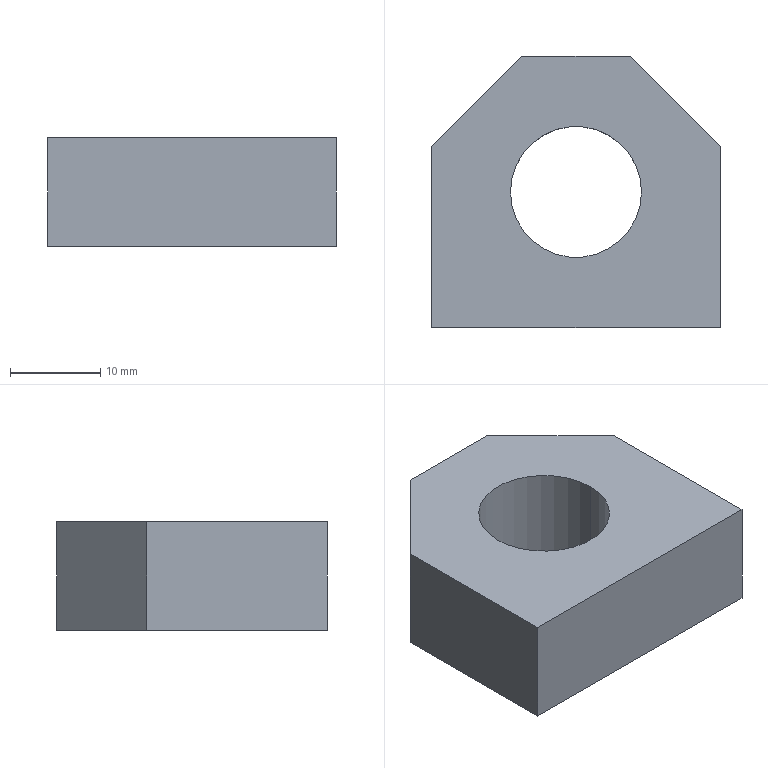Part | SolidWorks | features FlatPattern 1, SMBaseFlange 1, SheetMetal 1 | 1 solid | 10 faces | box 32 x 30 x 12 mm | volume 8338 mm3 | plane 8 | cylinder 2 | commonest cylinder face diameters 14.5 x2
STEP:
#1=CARTESIAN_POINT('',(8.75,15.,-12.));
#2=VERTEX_POINT('',#1);
#3=CARTESIAN_POINT('',(23.25,15.,-12.));
#4=VERTEX_POINT('',#3);
#5=CARTESIAN_POINT('',(16.,15.,-12.));
#6=DIRECTION('',(0.,0.,1.));
#7=DIRECTION('',(1.,0.,0.));
#8=AXIS2_PLACEMENT_3D('',#5,#6,#7);
#9=CIRCLE('',#8,7.25);
#10=EDGE_CURVE('',#2,#4,#9,.T.);
#11=ORIENTED_EDGE('',*,*,#10,.F.);
#12=CARTESIAN_POINT('',(8.75,15.,0.));
#13=VERTEX_POINT('',#12);
#14=CARTESIAN_POINT('',(8.75,15.,-12.));
#15=DIRECTION('',(0.,0.,1.));
#16=VECTOR('',#15,1000.);
#17=LINE('',#14,#16);
#18=EDGE_CURVE('',#2,#13,#17,.T.);
#19=ORIENTED_EDGE('',*,*,#18,.T.);
#20=CARTESIAN_POINT('',(23.25,15.,0.));
#21=VERTEX_POINT('',#20);
#22=CARTESIAN_POINT('',(16.,15.,0.));
#23=DIRECTION('',(0.,0.,1.));
#24=DIRECTION('',(1.,0.,0.));
#25=AXIS2_PLACEMENT_3D('',#22,#23,#24);
#26=CIRCLE('',#25,7.25);
#27=EDGE_CURVE('',#13,#21,#26,.T.);
#28=ORIENTED_EDGE('',*,*,#27,.T.);
#29=CARTESIAN_POINT('',(23.25,15.,-12.));
#30=DIRECTION('',(0.,0.,1.));
#31=VECTOR('',#30,1000.);
#32=LINE('',#29,#31);
#33=EDGE_CURVE('',#4,#21,#32,.T.);
#34=ORIENTED_EDGE('',*,*,#33,.F.);
#35=EDGE_LOOP('',(#11,#19,#28,#34));
#36=FACE_OUTER_BOUND('',#35,.T.);
#37=CARTESIAN_POINT('',(16.,15.,-12.));
#38=DIRECTION('',(0.,0.,1.));
#39=DIRECTION('',(1.,0.,0.));
#40=AXIS2_PLACEMENT_3D('',#37,#38,#39);
#41=CYLINDRICAL_SURFACE('',#40,7.25);
#42=ADVANCED_FACE('',(#36),#41,.F.);
#43=CARTESIAN_POINT('',(0.,20.,0.));
#44=VERTEX_POINT('',#43);
#45=CARTESIAN_POINT('',(0.,0.,0.));
#46=VERTEX_POINT('',#45);
#47=CARTESIAN_POINT('',(0.,0.,0.));
#48=DIRECTION('',(0.,-1.,0.));
#49=VECTOR('',#48,1000.);
#50=LINE('',#47,#49);
#51=EDGE_CURVE('',#44,#46,#50,.T.);
#52=ORIENTED_EDGE('',*,*,#51,.F.);
#53=CARTESIAN_POINT('',(0.,20.,-12.));
#54=VERTEX_POINT('',#53);
#55=CARTESIAN_POINT('',(0.,20.,-12.));
#56=DIRECTION('',(0.,0.,1.));
#57=VECTOR('',#56,1000.);
#58=LINE('',#55,#57);
#59=EDGE_CURVE('',#54,#44,#58,.T.);
#60=ORIENTED_EDGE('',*,*,#59,.F.);
#61=CARTESIAN_POINT('',(0.,0.,-12.));
#62=VERTEX_POINT('',#61);
#63=CARTESIAN_POINT('',(0.,0.,-12.));
#64=DIRECTION('',(0.,-1.,0.));
#65=VECTOR('',#64,1000.);
#66=LINE('',#63,#65);
#67=EDGE_CURVE('',#54,#62,#66,.T.);
#68=ORIENTED_EDGE('',*,*,#67,.T.);
#69=CARTESIAN_POINT('',(0.,0.,-12.));
#70=DIRECTION('',(0.,0.,1.));
#71=VECTOR('',#70,1000.);
#72=LINE('',#69,#71);
#73=EDGE_CURVE('',#62,#46,#72,.T.);
#74=ORIENTED_EDGE('',*,*,#73,.T.);
#75=EDGE_LOOP('',(#52,#60,#68,#74));
#76=FACE_OUTER_BOUND('',#75,.T.);
#77=CARTESIAN_POINT('',(0.,0.,-12.));
#78=DIRECTION('',(-1.,0.,0.));
#79=DIRECTION('',(0.,0.,1.));
#80=AXIS2_PLACEMENT_3D('',#77,#78,#79);
#81=PLANE('',#80);
#82=ADVANCED_FACE('',(#76),#81,.T.);
#83=CARTESIAN_POINT('',(10.,30.,0.));
#84=VERTEX_POINT('',#83);
#85=CARTESIAN_POINT('',(0.,20.,0.));
#86=DIRECTION('',(-0.7071,-0.7071,0.));
#87=VECTOR('',#86,1000.);
#88=LINE('',#85,#87);
#89=EDGE_CURVE('',#84,#44,#88,.T.);
#90=ORIENTED_EDGE('',*,*,#89,.F.);
#91=CARTESIAN_POINT('',(10.,30.,-12.));
#92=VERTEX_POINT('',#91);
#93=CARTESIAN_POINT('',(10.,30.,-12.));
#94=DIRECTION('',(0.,0.,1.));
#95=VECTOR('',#94,1000.);
#96=LINE('',#93,#95);
#97=EDGE_CURVE('',#92,#84,#96,.T.);
#98=ORIENTED_EDGE('',*,*,#97,.F.);
#99=CARTESIAN_POINT('',(0.,20.,-12.));
#100=DIRECTION('',(-0.7071,-0.7071,0.));
#101=VECTOR('',#100,1000.);
#102=LINE('',#99,#101);
#103=EDGE_CURVE('',#92,#54,#102,.T.);
#104=ORIENTED_EDGE('',*,*,#103,.T.);
#105=ORIENTED_EDGE('',*,*,#59,.T.);
#106=EDGE_LOOP('',(#90,#98,#104,#105));
#107=FACE_OUTER_BOUND('',#106,.T.);
#108=CARTESIAN_POINT('',(0.,20.,-12.));
#109=DIRECTION('',(-0.7071,0.7071,0.));
#110=DIRECTION('',(-0.7071,-0.7071,0.));
#111=AXIS2_PLACEMENT_3D('',#108,#109,#110);
#112=PLANE('',#111);
#113=ADVANCED_FACE('',(#107),#112,.T.);
#114=CARTESIAN_POINT('',(22.,30.,0.));
#115=VERTEX_POINT('',#114);
#116=CARTESIAN_POINT('',(10.,30.,0.));
#117=DIRECTION('',(-1.,0.,0.));
#118=VECTOR('',#117,1000.);
#119=LINE('',#116,#118);
#120=EDGE_CURVE('',#115,#84,#119,.T.);
#121=ORIENTED_EDGE('',*,*,#120,.F.);
#122=CARTESIAN_POINT('',(22.,30.,-12.));
#123=VERTEX_POINT('',#122);
#124=CARTESIAN_POINT('',(22.,30.,-12.));
#125=DIRECTION('',(0.,0.,1.));
#126=VECTOR('',#125,1000.);
#127=LINE('',#124,#126);
#128=EDGE_CURVE('',#123,#115,#127,.T.);
#129=ORIENTED_EDGE('',*,*,#128,.F.);
#130=CARTESIAN_POINT('',(10.,30.,-12.));
#131=DIRECTION('',(-1.,0.,0.));
#132=VECTOR('',#131,1000.);
#133=LINE('',#130,#132);
#134=EDGE_CURVE('',#123,#92,#133,.T.);
#135=ORIENTED_EDGE('',*,*,#134,.T.);
#136=ORIENTED_EDGE('',*,*,#97,.T.);
#137=EDGE_LOOP('',(#121,#129,#135,#136));
#138=FACE_OUTER_BOUND('',#137,.T.);
#139=CARTESIAN_POINT('',(10.,30.,-12.));
#140=DIRECTION('',(0.,1.,0.));
#141=DIRECTION('',(0.,0.,1.));
#142=AXIS2_PLACEMENT_3D('',#139,#140,#141);
#143=PLANE('',#142);
#144=ADVANCED_FACE('',(#138),#143,.T.);
#145=CARTESIAN_POINT('',(32.,20.,0.));
#146=VERTEX_POINT('',#145);
#147=CARTESIAN_POINT('',(22.,30.,0.));
#148=DIRECTION('',(-0.7071,0.7071,0.));
#149=VECTOR('',#148,1000.);
#150=LINE('',#147,#149);
#151=EDGE_CURVE('',#146,#115,#150,.T.);
#152=ORIENTED_EDGE('',*,*,#151,.F.);
#153=CARTESIAN_POINT('',(32.,20.,-12.));
#154=VERTEX_POINT('',#153);
#155=CARTESIAN_POINT('',(32.,20.,-12.));
#156=DIRECTION('',(0.,0.,1.));
#157=VECTOR('',#156,1000.);
#158=LINE('',#155,#157);
#159=EDGE_CURVE('',#154,#146,#158,.T.);
#160=ORIENTED_EDGE('',*,*,#159,.F.);
#161=CARTESIAN_POINT('',(22.,30.,-12.));
#162=DIRECTION('',(-0.7071,0.7071,0.));
#163=VECTOR('',#162,1000.);
#164=LINE('',#161,#163);
#165=EDGE_CURVE('',#154,#123,#164,.T.);
#166=ORIENTED_EDGE('',*,*,#165,.T.);
#167=ORIENTED_EDGE('',*,*,#128,.T.);
#168=EDGE_LOOP('',(#152,#160,#166,#167));
#169=FACE_OUTER_BOUND('',#168,.T.);
#170=CARTESIAN_POINT('',(22.,30.,-12.));
#171=DIRECTION('',(0.7071,0.7071,0.));
#172=DIRECTION('',(-0.7071,0.7071,0.));
#173=AXIS2_PLACEMENT_3D('',#170,#171,#172);
#174=PLANE('',#173);
#175=ADVANCED_FACE('',(#169),#174,.T.);
#176=CARTESIAN_POINT('',(32.,0.,0.));
#177=VERTEX_POINT('',#176);
#178=CARTESIAN_POINT('',(32.,0.,0.));
#179=DIRECTION('',(0.,1.,0.));
#180=VECTOR('',#179,1000.);
#181=LINE('',#178,#180);
#182=EDGE_CURVE('',#177,#146,#181,.T.);
#183=ORIENTED_EDGE('',*,*,#182,.F.);
#184=CARTESIAN_POINT('',(32.,0.,-12.));
#185=VERTEX_POINT('',#184);
#186=CARTESIAN_POINT('',(32.,0.,-12.));
#187=DIRECTION('',(0.,0.,1.));
#188=VECTOR('',#187,1000.);
#189=LINE('',#186,#188);
#190=EDGE_CURVE('',#185,#177,#189,.T.);
#191=ORIENTED_EDGE('',*,*,#190,.F.);
#192=CARTESIAN_POINT('',(32.,0.,-12.));
#193=DIRECTION('',(0.,1.,0.));
#194=VECTOR('',#193,1000.);
#195=LINE('',#192,#194);
#196=EDGE_CURVE('',#185,#154,#195,.T.);
#197=ORIENTED_EDGE('',*,*,#196,.T.);
#198=ORIENTED_EDGE('',*,*,#159,.T.);
#199=EDGE_LOOP('',(#183,#191,#197,#198));
#200=FACE_OUTER_BOUND('',#199,.T.);
#201=CARTESIAN_POINT('',(32.,0.,-12.));
#202=DIRECTION('',(1.,0.,0.));
#203=DIRECTION('',(0.,0.,-1.));
#204=AXIS2_PLACEMENT_3D('',#201,#202,#203);
#205=PLANE('',#204);
#206=ADVANCED_FACE('',(#200),#205,.T.);
#207=CARTESIAN_POINT('',(0.,0.,0.));
#208=DIRECTION('',(1.,0.,0.));
#209=VECTOR('',#208,1000.);
#210=LINE('',#207,#209);
#211=EDGE_CURVE('',#46,#177,#210,.T.);
#212=ORIENTED_EDGE('',*,*,#211,.F.);
#213=ORIENTED_EDGE('',*,*,#73,.F.);
#214=CARTESIAN_POINT('',(0.,0.,-12.));
#215=DIRECTION('',(1.,0.,0.));
#216=VECTOR('',#215,1000.);
#217=LINE('',#214,#216);
#218=EDGE_CURVE('',#62,#185,#217,.T.);
#219=ORIENTED_EDGE('',*,*,#218,.T.);
#220=ORIENTED_EDGE('',*,*,#190,.T.);
#221=EDGE_LOOP('',(#212,#213,#219,#220));
#222=FACE_OUTER_BOUND('',#221,.T.);
#223=CARTESIAN_POINT('',(0.,0.,-12.));
#224=DIRECTION('',(0.,-1.,0.));
#225=DIRECTION('',(0.,0.,-1.));
#226=AXIS2_PLACEMENT_3D('',#223,#224,#225);
#227=PLANE('',#226);
#228=ADVANCED_FACE('',(#222),#227,.T.);
#229=CARTESIAN_POINT('',(16.,15.,-12.));
#230=DIRECTION('',(0.,0.,1.));
#231=DIRECTION('',(1.,0.,0.));
#232=AXIS2_PLACEMENT_3D('',#229,#230,#231);
#233=CIRCLE('',#232,7.25);
#234=EDGE_CURVE('',#4,#2,#233,.T.);
#235=ORIENTED_EDGE('',*,*,#234,.T.);
#236=ORIENTED_EDGE('',*,*,#10,.T.);
#237=EDGE_LOOP('',(#235,#236));
#238=FACE_BOUND('',#237,.T.);
#239=ORIENTED_EDGE('',*,*,#67,.F.);
#240=ORIENTED_EDGE('',*,*,#103,.F.);
#241=ORIENTED_EDGE('',*,*,#134,.F.);
#242=ORIENTED_EDGE('',*,*,#165,.F.);
#243=ORIENTED_EDGE('',*,*,#196,.F.);
#244=ORIENTED_EDGE('',*,*,#218,.F.);
#245=EDGE_LOOP('',(#239,#240,#241,#242,#243,#244));
#246=FACE_OUTER_BOUND('',#245,.T.);
#247=CARTESIAN_POINT('',(0.,0.,-12.));
#248=DIRECTION('',(0.,0.,-1.));
#249=DIRECTION('',(-1.,0.,0.));
#250=AXIS2_PLACEMENT_3D('',#247,#248,#249);
#251=PLANE('',#250);
#252=ADVANCED_FACE('',(#238,#246),#251,.T.);
#253=CARTESIAN_POINT('',(16.,15.,0.));
#254=DIRECTION('',(0.,0.,1.));
#255=DIRECTION('',(1.,0.,0.));
#256=AXIS2_PLACEMENT_3D('',#253,#254,#255);
#257=CIRCLE('',#256,7.25);
#258=EDGE_CURVE('',#21,#13,#257,.T.);
#259=ORIENTED_EDGE('',*,*,#258,.F.);
#260=ORIENTED_EDGE('',*,*,#27,.F.);
#261=EDGE_LOOP('',(#259,#260));
#262=FACE_BOUND('',#261,.T.);
#263=ORIENTED_EDGE('',*,*,#51,.T.);
#264=ORIENTED_EDGE('',*,*,#211,.T.);
#265=ORIENTED_EDGE('',*,*,#182,.T.);
#266=ORIENTED_EDGE('',*,*,#151,.T.);
#267=ORIENTED_EDGE('',*,*,#120,.T.);
#268=ORIENTED_EDGE('',*,*,#89,.T.);
#269=EDGE_LOOP('',(#263,#264,#265,#266,#267,#268));
#270=FACE_OUTER_BOUND('',#269,.T.);
#271=CARTESIAN_POINT('',(0.,0.,0.));
#272=DIRECTION('',(0.,0.,-1.));
#273=DIRECTION('',(-1.,0.,0.));
#274=AXIS2_PLACEMENT_3D('',#271,#272,#273);
#275=PLANE('',#274);
#276=ADVANCED_FACE('',(#262,#270),#275,.F.);
#277=ORIENTED_EDGE('',*,*,#18,.F.);
#278=ORIENTED_EDGE('',*,*,#234,.F.);
#279=ORIENTED_EDGE('',*,*,#33,.T.);
#280=ORIENTED_EDGE('',*,*,#258,.T.);
#281=EDGE_LOOP('',(#277,#278,#279,#280));
#282=FACE_OUTER_BOUND('',#281,.T.);
#283=CARTESIAN_POINT('',(16.,15.,-12.));
#284=DIRECTION('',(0.,0.,1.));
#285=DIRECTION('',(1.,0.,0.));
#286=AXIS2_PLACEMENT_3D('',#283,#284,#285);
#287=CYLINDRICAL_SURFACE('',#286,7.25);
#288=ADVANCED_FACE('',(#282),#287,.F.);
#289=CLOSED_SHELL('',(#42,#82,#113,#144,#175,#206,#228,#252,#276,#288));
#290=MANIFOLD_SOLID_BREP('',#289);
#291=CARTESIAN_POINT('',(0.,0.,0.));
#292=DIRECTION('',(0.,0.,1.));
#293=DIRECTION('',(1.,0.,0.));
#294=AXIS2_PLACEMENT_3D('',#291,#292,#293);
#295=(LENGTH_UNIT()NAMED_UNIT(*)SI_UNIT(.MILLI.,.METRE.));
#296=UNCERTAINTY_MEASURE_WITH_UNIT(LENGTH_MEASURE(0.00001),#295,'','');
#297=(NAMED_UNIT(*)PLANE_ANGLE_UNIT()SI_UNIT($,.RADIAN.));
#298=(NAMED_UNIT(*)SI_UNIT($,.STERADIAN.)SOLID_ANGLE_UNIT());
#299=(GEOMETRIC_REPRESENTATION_CONTEXT(3)GLOBAL_UNCERTAINTY_ASSIGNED_CONTEXT((#296))GLOBAL_UNIT_ASSIGNED_CONTEXT((#295,#297,#298))REPRESENTATION_CONTEXT('',''));
#300=ADVANCED_BREP_SHAPE_REPRESENTATION('',(#290,#294),#299);